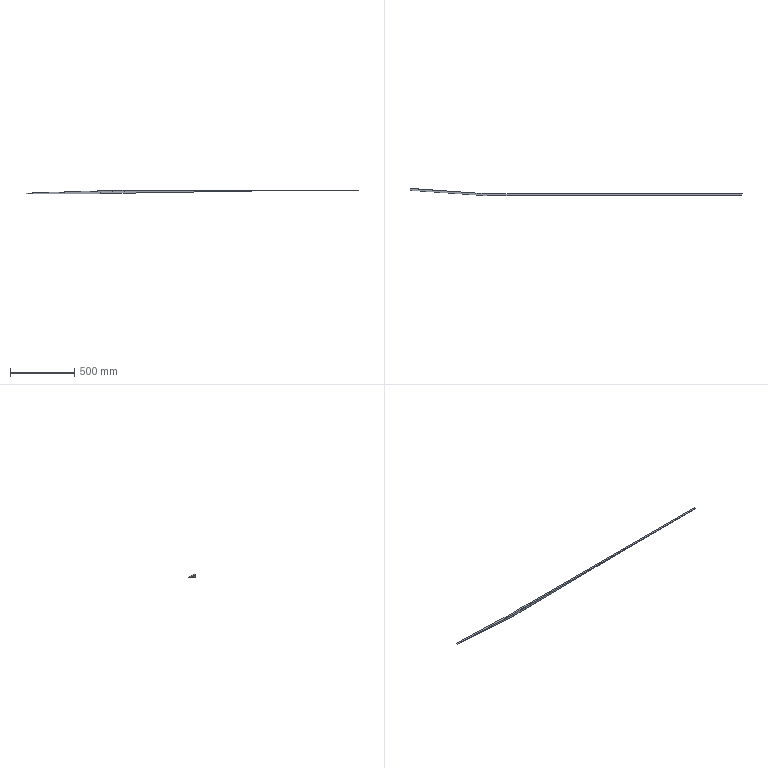Part | SolidWorks | features BaseBody 1 | 1 solid | 26 faces | box 2582 x 55.656 x 24.973 mm | volume 180184 mm3 | plane 26
STEP:
#1=CARTESIAN_POINT('',(2000.,-38.142,-0.6658));
#2=VERTEX_POINT('',#1);
#3=CARTESIAN_POINT('',(180.519,-38.128,-1.466));
#4=VERTEX_POINT('',#3);
#5=CARTESIAN_POINT('',(2000.,-38.142,-0.6658));
#6=DIRECTION('',(-1.,0.000007674,-0.0004396));
#7=VECTOR('',#6,1000.);
#8=LINE('',#5,#7);
#9=EDGE_CURVE('',#2,#4,#8,.T.);
#10=ORIENTED_EDGE('',*,*,#9,.F.);
#11=CARTESIAN_POINT('',(2000.,-23.141,-0.4373));
#12=VERTEX_POINT('',#11);
#13=CARTESIAN_POINT('',(2000.,-23.141,-0.4373));
#14=DIRECTION('',(-0.000000977,-0.9999,-0.01523));
#15=VECTOR('',#14,1000.);
#16=LINE('',#13,#15);
#17=EDGE_CURVE('',#12,#2,#16,.T.);
#18=ORIENTED_EDGE('',*,*,#17,.F.);
#19=CARTESIAN_POINT('',(180.519,-23.127,-1.237));
#20=VERTEX_POINT('',#19);
#21=CARTESIAN_POINT('',(180.519,-23.127,-1.237));
#22=DIRECTION('',(1.,-0.000007674,0.0004396));
#23=VECTOR('',#22,1000.);
#24=LINE('',#21,#23);
#25=EDGE_CURVE('',#20,#12,#24,.T.);
#26=ORIENTED_EDGE('',*,*,#25,.F.);
#27=CARTESIAN_POINT('',(180.519,-23.127,-1.237));
#28=DIRECTION('',(0.,0.9999,0.01523));
#29=VECTOR('',#28,1000.);
#30=LINE('',#27,#29);
#31=EDGE_CURVE('',#4,#20,#30,.T.);
#32=ORIENTED_EDGE('',*,*,#31,.F.);
#33=EDGE_LOOP('',(#10,#18,#26,#32));
#34=FACE_OUTER_BOUND('',#33,.T.);
#35=CARTESIAN_POINT('',(169.602,-38.22,-1.472));
#36=DIRECTION('',(0.0004397,0.01523,-0.9999));
#37=DIRECTION('',(0.,0.9999,0.01523));
#38=AXIS2_PLACEMENT_3D('',#35,#36,#37);
#39=PLANE('',#38);
#40=ADVANCED_FACE('',(#34),#39,.F.);
#41=CARTESIAN_POINT('',(90.17,-23.127,-1.237));
#42=VERTEX_POINT('',#41);
#43=CARTESIAN_POINT('',(135.344,-23.127,-1.237));
#44=DIRECTION('',(-1.,0.,0.));
#45=VECTOR('',#44,1000.);
#46=LINE('',#43,#45);
#47=EDGE_CURVE('',#20,#42,#46,.T.);
#48=ORIENTED_EDGE('',*,*,#47,.T.);
#49=CARTESIAN_POINT('',(90.17,-38.128,-1.466));
#50=VERTEX_POINT('',#49);
#51=CARTESIAN_POINT('',(90.17,-23.127,-1.237));
#52=DIRECTION('',(-0.00001304,-0.9999,-0.01523));
#53=VECTOR('',#52,1000.);
#54=LINE('',#51,#53);
#55=EDGE_CURVE('',#42,#50,#54,.T.);
#56=ORIENTED_EDGE('',*,*,#55,.T.);
#57=CARTESIAN_POINT('',(135.344,-38.128,-1.466));
#58=DIRECTION('',(1.,0.,0.));
#59=VECTOR('',#58,1000.);
#60=LINE('',#57,#59);
#61=EDGE_CURVE('',#50,#4,#60,.T.);
#62=ORIENTED_EDGE('',*,*,#61,.T.);
#63=ORIENTED_EDGE('',*,*,#31,.T.);
#64=EDGE_LOOP('',(#48,#56,#62,#63));
#65=FACE_OUTER_BOUND('',#64,.T.);
#66=CARTESIAN_POINT('',(89.628,-23.127,-1.237));
#67=DIRECTION('',(0.,-0.01523,0.9999));
#68=DIRECTION('',(0.,-0.9999,-0.01523));
#69=AXIS2_PLACEMENT_3D('',#66,#67,#68);
#70=PLANE('',#69);
#71=ADVANCED_FACE('',(#65),#70,.T.);
#72=CARTESIAN_POINT('',(180.528,-37.811,-22.266));
#73=VERTEX_POINT('',#72);
#74=CARTESIAN_POINT('',(180.519,-38.128,-1.466));
#75=DIRECTION('',(0.0004397,0.01523,-0.9999));
#76=VECTOR('',#75,1000.);
#77=LINE('',#74,#76);
#78=EDGE_CURVE('',#4,#73,#77,.T.);
#79=ORIENTED_EDGE('',*,*,#78,.T.);
#80=CARTESIAN_POINT('',(1223.587,-38.087,-4.207));
#81=VERTEX_POINT('',#80);
#82=CARTESIAN_POINT('',(180.528,-37.811,-22.266));
#83=DIRECTION('',(0.9999,-0.0002647,0.01731));
#84=VECTOR('',#83,1000.);
#85=LINE('',#82,#84);
#86=EDGE_CURVE('',#73,#81,#85,.T.);
#87=ORIENTED_EDGE('',*,*,#86,.T.);
#88=CARTESIAN_POINT('',(2000.001,-38.093,-3.865));
#89=VERTEX_POINT('',#88);
#90=CARTESIAN_POINT('',(1223.587,-38.087,-4.207));
#91=DIRECTION('',(1.,-0.000007674,0.0004396));
#92=VECTOR('',#91,1000.);
#93=LINE('',#90,#92);
#94=EDGE_CURVE('',#81,#89,#93,.T.);
#95=ORIENTED_EDGE('',*,*,#94,.T.);
#96=CARTESIAN_POINT('',(2000.001,-38.093,-3.865));
#97=DIRECTION('',(-0.0004395,-0.01523,0.9999));
#98=VECTOR('',#97,1000.);
#99=LINE('',#96,#98);
#100=EDGE_CURVE('',#89,#2,#99,.T.);
#101=ORIENTED_EDGE('',*,*,#100,.T.);
#102=ORIENTED_EDGE('',*,*,#9,.T.);
#103=EDGE_LOOP('',(#79,#87,#95,#101,#102));
#104=FACE_OUTER_BOUND('',#103,.T.);
#105=CARTESIAN_POINT('',(180.519,-38.14,-0.6657));
#106=DIRECTION('',(-0.000000977,-0.9999,-0.01523));
#107=DIRECTION('',(0.,0.01523,-0.9999));
#108=AXIS2_PLACEMENT_3D('',#105,#106,#107);
#109=PLANE('',#108);
#110=ADVANCED_FACE('',(#104),#109,.T.);
#111=CARTESIAN_POINT('',(2000.001,-23.092,-3.637));
#112=VERTEX_POINT('',#111);
#113=CARTESIAN_POINT('',(2000.001,-23.092,-3.637));
#114=DIRECTION('',(-0.0004397,-0.01523,0.9999));
#115=VECTOR('',#114,1000.);
#116=LINE('',#113,#115);
#117=EDGE_CURVE('',#112,#12,#116,.T.);
#118=ORIENTED_EDGE('',*,*,#117,.T.);
#119=ORIENTED_EDGE('',*,*,#17,.T.);
#120=ORIENTED_EDGE('',*,*,#100,.F.);
#121=CARTESIAN_POINT('',(2000.001,-38.093,-3.865));
#122=DIRECTION('',(0.000000977,0.9999,0.01523));
#123=VECTOR('',#122,1000.);
#124=LINE('',#121,#123);
#125=EDGE_CURVE('',#89,#112,#124,.T.);
#126=ORIENTED_EDGE('',*,*,#125,.T.);
#127=EDGE_LOOP('',(#118,#119,#120,#126));
#128=FACE_OUTER_BOUND('',#127,.T.);
#129=CARTESIAN_POINT('',(2000.,-38.232,-0.4167));
#130=DIRECTION('',(1.,-0.000007674,0.0004396));
#131=DIRECTION('',(0.0004396,0.,-1.));
#132=AXIS2_PLACEMENT_3D('',#129,#130,#131);
#133=PLANE('',#132);
#134=ADVANCED_FACE('',(#128),#133,.T.);
#135=ORIENTED_EDGE('',*,*,#117,.F.);
#136=CARTESIAN_POINT('',(180.52,-23.079,-4.437));
#137=VERTEX_POINT('',#136);
#138=CARTESIAN_POINT('',(2000.001,-23.092,-3.637));
#139=DIRECTION('',(-1.,0.000007674,-0.0004396));
#140=VECTOR('',#139,1000.);
#141=LINE('',#138,#140);
#142=EDGE_CURVE('',#112,#137,#141,.T.);
#143=ORIENTED_EDGE('',*,*,#142,.T.);
#144=CARTESIAN_POINT('',(180.52,-23.079,-4.437));
#145=DIRECTION('',(-0.0004396,-0.01523,0.9999));
#146=VECTOR('',#145,1000.);
#147=LINE('',#144,#146);
#148=EDGE_CURVE('',#137,#20,#147,.T.);
#149=ORIENTED_EDGE('',*,*,#148,.T.);
#150=ORIENTED_EDGE('',*,*,#25,.T.);
#151=EDGE_LOOP('',(#135,#143,#149,#150));
#152=FACE_OUTER_BOUND('',#151,.T.);
#153=CARTESIAN_POINT('',(169.602,-23.078,-4.461));
#154=DIRECTION('',(0.000000977,0.9999,0.01523));
#155=DIRECTION('',(0.,-0.01523,0.9999));
#156=AXIS2_PLACEMENT_3D('',#153,#154,#155);
#157=PLANE('',#156);
#158=ADVANCED_FACE('',(#152),#157,.T.);
#159=CARTESIAN_POINT('',(-5.976,-23.078,-4.291));
#160=VERTEX_POINT('',#159);
#161=CARTESIAN_POINT('',(-5.976,-23.078,-4.291));
#162=DIRECTION('',(0.9995,-0.0005096,0.03174));
#163=VECTOR('',#162,1000.);
#164=LINE('',#161,#163);
#165=EDGE_CURVE('',#160,#42,#164,.T.);
#166=ORIENTED_EDGE('',*,*,#165,.F.);
#167=CARTESIAN_POINT('',(-6.5,-38.079,-4.536));
#168=VERTEX_POINT('',#167);
#169=CARTESIAN_POINT('',(-6.5,-38.079,-4.536));
#170=DIRECTION('',(0.03491,0.9993,0.01633));
#171=VECTOR('',#170,1000.);
#172=LINE('',#169,#171);
#173=EDGE_CURVE('',#168,#160,#172,.T.);
#174=ORIENTED_EDGE('',*,*,#173,.F.);
#175=CARTESIAN_POINT('',(90.17,-38.128,-1.466));
#176=DIRECTION('',(-0.9995,0.0005096,-0.03174));
#177=VECTOR('',#176,1000.);
#178=LINE('',#175,#177);
#179=EDGE_CURVE('',#50,#168,#178,.T.);
#180=ORIENTED_EDGE('',*,*,#179,.F.);
#181=ORIENTED_EDGE('',*,*,#55,.F.);
#182=EDGE_LOOP('',(#166,#174,#180,#181));
#183=FACE_OUTER_BOUND('',#182,.T.);
#184=CARTESIAN_POINT('',(90.758,-38.218,-1.448));
#185=DIRECTION('',(0.03175,0.01522,-0.9994));
#186=DIRECTION('',(-0.9995,0.,-0.03175));
#187=AXIS2_PLACEMENT_3D('',#184,#185,#186);
#188=PLANE('',#187);
#189=ADVANCED_FACE('',(#183),#188,.F.);
#190=CARTESIAN_POINT('',(90.221,-23.079,-4.437));
#191=VERTEX_POINT('',#190);
#192=CARTESIAN_POINT('',(135.345,-23.079,-4.437));
#193=DIRECTION('',(1.,0.,0.));
#194=VECTOR('',#193,1000.);
#195=LINE('',#192,#194);
#196=EDGE_CURVE('',#191,#137,#195,.T.);
#197=ORIENTED_EDGE('',*,*,#196,.F.);
#198=CARTESIAN_POINT('',(90.17,-23.127,-1.237));
#199=DIRECTION('',(0.01588,0.01523,-0.9998));
#200=VECTOR('',#199,1000.);
#201=LINE('',#198,#200);
#202=EDGE_CURVE('',#42,#191,#201,.T.);
#203=ORIENTED_EDGE('',*,*,#202,.F.);
#204=ORIENTED_EDGE('',*,*,#47,.F.);
#205=ORIENTED_EDGE('',*,*,#148,.F.);
#206=EDGE_LOOP('',(#197,#203,#204,#205));
#207=FACE_OUTER_BOUND('',#206,.T.);
#208=CARTESIAN_POINT('',(89.628,-23.127,-1.237));
#209=DIRECTION('',(0.,-0.9999,-0.01523));
#210=DIRECTION('',(0.,0.01523,-0.9999));
#211=AXIS2_PLACEMENT_3D('',#208,#209,#210);
#212=PLANE('',#211);
#213=ADVANCED_FACE('',(#207),#212,.F.);
#214=ORIENTED_EDGE('',*,*,#61,.F.);
#215=CARTESIAN_POINT('',(90.5,-37.811,-22.266));
#216=VERTEX_POINT('',#215);
#217=CARTESIAN_POINT('',(90.5,-37.811,-22.266));
#218=DIRECTION('',(-0.01588,-0.01523,0.9998));
#219=VECTOR('',#218,1000.);
#220=LINE('',#217,#219);
#221=EDGE_CURVE('',#216,#50,#220,.T.);
#222=ORIENTED_EDGE('',*,*,#221,.F.);
#223=CARTESIAN_POINT('',(135.349,-37.811,-22.266));
#224=DIRECTION('',(-1.,0.,0.));
#225=VECTOR('',#224,1000.);
#226=LINE('',#223,#225);
#227=EDGE_CURVE('',#73,#216,#226,.T.);
#228=ORIENTED_EDGE('',*,*,#227,.F.);
#229=ORIENTED_EDGE('',*,*,#78,.F.);
#230=EDGE_LOOP('',(#214,#222,#228,#229));
#231=FACE_OUTER_BOUND('',#230,.T.);
#232=CARTESIAN_POINT('',(89.628,-37.811,-22.266));
#233=DIRECTION('',(0.,0.9999,0.01523));
#234=DIRECTION('',(0.,-0.01523,0.9999));
#235=AXIS2_PLACEMENT_3D('',#232,#233,#234);
#236=PLANE('',#235);
#237=ADVANCED_FACE('',(#231),#236,.F.);
#238=CARTESIAN_POINT('',(180.528,-34.611,-22.218));
#239=VERTEX_POINT('',#238);
#240=CARTESIAN_POINT('',(180.528,-37.811,-22.266));
#241=DIRECTION('',(0.,-0.9999,-0.01523));
#242=VECTOR('',#241,1000.);
#243=LINE('',#240,#242);
#244=EDGE_CURVE('',#239,#73,#243,.T.);
#245=ORIENTED_EDGE('',*,*,#244,.F.);
#246=CARTESIAN_POINT('',(1223.587,-34.887,-4.158));
#247=VERTEX_POINT('',#246);
#248=CARTESIAN_POINT('',(1223.587,-34.887,-4.158));
#249=DIRECTION('',(-0.9999,0.0002647,-0.01731));
#250=VECTOR('',#249,1000.);
#251=LINE('',#248,#250);
#252=EDGE_CURVE('',#247,#239,#251,.T.);
#253=ORIENTED_EDGE('',*,*,#252,.F.);
#254=CARTESIAN_POINT('',(1223.587,-38.088,-4.207));
#255=DIRECTION('',(0.,0.9999,0.01523));
#256=VECTOR('',#255,1000.);
#257=LINE('',#254,#256);
#258=EDGE_CURVE('',#81,#247,#257,.T.);
#259=ORIENTED_EDGE('',*,*,#258,.F.);
#260=ORIENTED_EDGE('',*,*,#86,.F.);
#261=EDGE_LOOP('',(#245,#253,#259,#260));
#262=FACE_OUTER_BOUND('',#261,.T.);
#263=CARTESIAN_POINT('',(174.27,-38.108,-22.379));
#264=DIRECTION('',(-0.01731,-0.01523,0.9997));
#265=DIRECTION('',(0.9999,0.,0.01732));
#266=AXIS2_PLACEMENT_3D('',#263,#264,#265);
#267=PLANE('',#266);
#268=ADVANCED_FACE('',(#262),#267,.F.);
#269=ORIENTED_EDGE('',*,*,#258,.T.);
#270=CARTESIAN_POINT('',(180.52,-34.879,-4.617));
#271=VERTEX_POINT('',#270);
#272=CARTESIAN_POINT('',(1223.587,-34.887,-4.158));
#273=DIRECTION('',(-1.,0.000007674,-0.0004396));
#274=VECTOR('',#273,1000.);
#275=LINE('',#272,#274);
#276=EDGE_CURVE('',#247,#271,#275,.T.);
#277=ORIENTED_EDGE('',*,*,#276,.T.);
#278=CARTESIAN_POINT('',(180.52,-38.081,-4.665));
#279=DIRECTION('',(0.,0.9999,0.01523));
#280=VECTOR('',#279,1000.);
#281=LINE('',#278,#280);
#282=EDGE_CURVE('',#271,#137,#281,.T.);
#283=ORIENTED_EDGE('',*,*,#282,.T.);
#284=ORIENTED_EDGE('',*,*,#142,.F.);
#285=ORIENTED_EDGE('',*,*,#125,.F.);
#286=ORIENTED_EDGE('',*,*,#94,.F.);
#287=EDGE_LOOP('',(#269,#277,#283,#284,#285,#286));
#288=FACE_OUTER_BOUND('',#287,.T.);
#289=CARTESIAN_POINT('',(180.52,-38.081,-4.665));
#290=DIRECTION('',(0.0004397,0.01523,-0.9999));
#291=DIRECTION('',(0.,0.9999,0.01523));
#292=AXIS2_PLACEMENT_3D('',#289,#290,#291);
#293=PLANE('',#292);
#294=ADVANCED_FACE('',(#288),#293,.T.);
#295=CARTESIAN_POINT('',(-5.875,-23.03,-7.489));
#296=VERTEX_POINT('',#295);
#297=CARTESIAN_POINT('',(90.221,-23.079,-4.437));
#298=DIRECTION('',(-0.9995,0.0005096,-0.03174));
#299=VECTOR('',#298,1000.);
#300=LINE('',#297,#299);
#301=EDGE_CURVE('',#191,#296,#300,.T.);
#302=ORIENTED_EDGE('',*,*,#301,.T.);
#303=CARTESIAN_POINT('',(-5.875,-23.03,-7.489));
#304=DIRECTION('',(-0.03175,-0.01522,0.9994));
#305=VECTOR('',#304,1000.);
#306=LINE('',#303,#305);
#307=EDGE_CURVE('',#296,#160,#306,.T.);
#308=ORIENTED_EDGE('',*,*,#307,.T.);
#309=ORIENTED_EDGE('',*,*,#165,.T.);
#310=ORIENTED_EDGE('',*,*,#202,.T.);
#311=EDGE_LOOP('',(#302,#308,#309,#310));
#312=FACE_OUTER_BOUND('',#311,.T.);
#313=CARTESIAN_POINT('',(-6.554,-23.029,-7.526));
#314=DIRECTION('',(0.00002607,0.9999,0.01523));
#315=DIRECTION('',(0.,-0.01523,0.9999));
#316=AXIS2_PLACEMENT_3D('',#313,#314,#315);
#317=PLANE('',#316);
#318=ADVANCED_FACE('',(#312),#317,.T.);
#319=CARTESIAN_POINT('',(-581.281,17.465,-21.951));
#320=VERTEX_POINT('',#319);
#321=CARTESIAN_POINT('',(-5.976,-23.078,-4.291));
#322=DIRECTION('',(-0.9971,0.07027,-0.03061));
#323=VECTOR('',#322,1000.);
#324=LINE('',#321,#323);
#325=EDGE_CURVE('',#160,#320,#324,.T.);
#326=ORIENTED_EDGE('',*,*,#325,.T.);
#327=CARTESIAN_POINT('',(-582.328,2.502,-22.213));
#328=VERTEX_POINT('',#327);
#329=CARTESIAN_POINT('',(-581.281,17.465,-21.951));
#330=DIRECTION('',(-0.06976,-0.9974,-0.01741));
#331=VECTOR('',#330,1000.);
#332=LINE('',#329,#331);
#333=EDGE_CURVE('',#320,#328,#332,.T.);
#334=ORIENTED_EDGE('',*,*,#333,.T.);
#335=CARTESIAN_POINT('',(-582.328,2.502,-22.213));
#336=DIRECTION('',(0.9971,-0.07027,0.03061));
#337=VECTOR('',#336,1000.);
#338=LINE('',#335,#337);
#339=EDGE_CURVE('',#328,#168,#338,.T.);
#340=ORIENTED_EDGE('',*,*,#339,.T.);
#341=ORIENTED_EDGE('',*,*,#173,.T.);
#342=EDGE_LOOP('',(#326,#334,#340,#341));
#343=FACE_OUTER_BOUND('',#342,.T.);
#344=CARTESIAN_POINT('',(-585.766,-38.412,-22.945));
#345=DIRECTION('',(-0.03175,-0.01522,0.9994));
#346=DIRECTION('',(0.9995,0.,0.03176));
#347=AXIS2_PLACEMENT_3D('',#344,#345,#346);
#348=PLANE('',#347);
#349=ADVANCED_FACE('',(#343),#348,.T.);
#350=ORIENTED_EDGE('',*,*,#179,.T.);
#351=CARTESIAN_POINT('',(-5.84,-37.762,-25.326));
#352=VERTEX_POINT('',#351);
#353=CARTESIAN_POINT('',(-6.5,-38.079,-4.536));
#354=DIRECTION('',(0.03175,0.01522,-0.9994));
#355=VECTOR('',#354,1000.);
#356=LINE('',#353,#355);
#357=EDGE_CURVE('',#168,#352,#356,.T.);
#358=ORIENTED_EDGE('',*,*,#357,.T.);
#359=CARTESIAN_POINT('',(-5.84,-37.762,-25.326));
#360=DIRECTION('',(0.9995,-0.0005096,0.03174));
#361=VECTOR('',#360,1000.);
#362=LINE('',#359,#361);
#363=EDGE_CURVE('',#352,#216,#362,.T.);
#364=ORIENTED_EDGE('',*,*,#363,.T.);
#365=ORIENTED_EDGE('',*,*,#221,.T.);
#366=EDGE_LOOP('',(#350,#358,#364,#365));
#367=FACE_OUTER_BOUND('',#366,.T.);
#368=CARTESIAN_POINT('',(-7.082,-38.127,-1.322));
#369=DIRECTION('',(-0.00002607,-0.9999,-0.01523));
#370=DIRECTION('',(0.,0.01523,-0.9999));
#371=AXIS2_PLACEMENT_3D('',#368,#369,#370);
#372=PLANE('',#371);
#373=ADVANCED_FACE('',(#367),#372,.T.);
#374=CARTESIAN_POINT('',(90.221,-34.879,-4.617));
#375=VERTEX_POINT('',#374);
#376=CARTESIAN_POINT('',(135.371,-34.879,-4.617));
#377=DIRECTION('',(1.,0.,0.));
#378=VECTOR('',#377,1000.);
#379=LINE('',#376,#378);
#380=EDGE_CURVE('',#375,#271,#379,.T.);
#381=ORIENTED_EDGE('',*,*,#380,.F.);
#382=CARTESIAN_POINT('',(90.221,-23.079,-4.437));
#383=DIRECTION('',(-0.00001304,-0.9999,-0.01523));
#384=VECTOR('',#383,1000.);
#385=LINE('',#382,#384);
#386=EDGE_CURVE('',#191,#375,#385,.T.);
#387=ORIENTED_EDGE('',*,*,#386,.F.);
#388=ORIENTED_EDGE('',*,*,#196,.T.);
#389=ORIENTED_EDGE('',*,*,#282,.F.);
#390=EDGE_LOOP('',(#381,#387,#388,#389));
#391=FACE_OUTER_BOUND('',#390,.T.);
#392=CARTESIAN_POINT('',(89.679,-23.079,-4.437));
#393=DIRECTION('',(0.,-0.01523,0.9999));
#394=DIRECTION('',(0.,-0.9999,-0.01523));
#395=AXIS2_PLACEMENT_3D('',#392,#393,#394);
#396=PLANE('',#395);
#397=ADVANCED_FACE('',(#391),#396,.F.);
#398=ORIENTED_EDGE('',*,*,#227,.T.);
#399=CARTESIAN_POINT('',(90.5,-34.611,-22.218));
#400=VERTEX_POINT('',#399);
#401=CARTESIAN_POINT('',(90.5,-37.811,-22.266));
#402=DIRECTION('',(0.00001302,0.9999,0.01523));
#403=VECTOR('',#402,1000.);
#404=LINE('',#401,#403);
#405=EDGE_CURVE('',#216,#400,#404,.T.);
#406=ORIENTED_EDGE('',*,*,#405,.T.);
#407=CARTESIAN_POINT('',(135.244,-34.611,-22.218));
#408=DIRECTION('',(1.,0.,0.));
#409=VECTOR('',#408,1000.);
#410=LINE('',#407,#409);
#411=EDGE_CURVE('',#400,#239,#410,.T.);
#412=ORIENTED_EDGE('',*,*,#411,.T.);
#413=ORIENTED_EDGE('',*,*,#244,.T.);
#414=EDGE_LOOP('',(#398,#406,#412,#413));
#415=FACE_OUTER_BOUND('',#414,.T.);
#416=CARTESIAN_POINT('',(89.96,-37.811,-22.266));
#417=DIRECTION('',(0.,0.01523,-0.9999));
#418=DIRECTION('',(0.,0.9999,0.01523));
#419=AXIS2_PLACEMENT_3D('',#416,#417,#418);
#420=PLANE('',#419);
#421=ADVANCED_FACE('',(#415),#420,.T.);
#422=ORIENTED_EDGE('',*,*,#252,.T.);
#423=CARTESIAN_POINT('',(180.52,-34.879,-4.617));
#424=DIRECTION('',(0.0004397,0.01523,-0.9999));
#425=VECTOR('',#424,1000.);
#426=LINE('',#423,#425);
#427=EDGE_CURVE('',#271,#239,#426,.T.);
#428=ORIENTED_EDGE('',*,*,#427,.F.);
#429=ORIENTED_EDGE('',*,*,#276,.F.);
#430=EDGE_LOOP('',(#422,#428,#429));
#431=FACE_OUTER_BOUND('',#430,.T.);
#432=CARTESIAN_POINT('',(174.262,-34.888,-4.05));
#433=DIRECTION('',(-0.000000977,-0.9999,-0.01523));
#434=DIRECTION('',(0.,0.01523,-0.9999));
#435=AXIS2_PLACEMENT_3D('',#432,#433,#434);
#436=PLANE('',#435);
#437=ADVANCED_FACE('',(#431),#436,.F.);
#438=CARTESIAN_POINT('',(-581.18,17.514,-25.149));
#439=VERTEX_POINT('',#438);
#440=CARTESIAN_POINT('',(-581.18,17.514,-25.149));
#441=DIRECTION('',(0.9971,-0.07027,0.03061));
#442=VECTOR('',#441,1000.);
#443=LINE('',#440,#442);
#444=EDGE_CURVE('',#439,#296,#443,.T.);
#445=ORIENTED_EDGE('',*,*,#444,.F.);
#446=CARTESIAN_POINT('',(-581.281,17.465,-21.951));
#447=DIRECTION('',(0.03175,0.01522,-0.9994));
#448=VECTOR('',#447,1000.);
#449=LINE('',#446,#448);
#450=EDGE_CURVE('',#320,#439,#449,.T.);
#451=ORIENTED_EDGE('',*,*,#450,.F.);
#452=ORIENTED_EDGE('',*,*,#325,.F.);
#453=ORIENTED_EDGE('',*,*,#307,.F.);
#454=EDGE_LOOP('',(#445,#451,#452,#453));
#455=FACE_OUTER_BOUND('',#454,.T.);
#456=CARTESIAN_POINT('',(-584.73,17.765,-25.275));
#457=DIRECTION('',(-0.06976,-0.9974,-0.01741));
#458=DIRECTION('',(0.9976,-0.06977,0.));
#459=AXIS2_PLACEMENT_3D('',#456,#457,#458);
#460=PLANE('',#459);
#461=ADVANCED_FACE('',(#455),#460,.F.);
#462=CARTESIAN_POINT('',(-6.287,-34.83,-7.681));
#463=VERTEX_POINT('',#462);
#464=CARTESIAN_POINT('',(90.221,-34.879,-4.617));
#465=DIRECTION('',(-0.9995,0.0005096,-0.03174));
#466=VECTOR('',#465,1000.);
#467=LINE('',#464,#466);
#468=EDGE_CURVE('',#375,#463,#467,.T.);
#469=ORIENTED_EDGE('',*,*,#468,.T.);
#470=CARTESIAN_POINT('',(-6.287,-34.83,-7.681));
#471=DIRECTION('',(0.03491,0.9993,0.01633));
#472=VECTOR('',#471,1000.);
#473=LINE('',#470,#472);
#474=EDGE_CURVE('',#463,#296,#473,.T.);
#475=ORIENTED_EDGE('',*,*,#474,.T.);
#476=ORIENTED_EDGE('',*,*,#301,.F.);
#477=ORIENTED_EDGE('',*,*,#386,.T.);
#478=EDGE_LOOP('',(#469,#475,#476,#477));
#479=FACE_OUTER_BOUND('',#478,.T.);
#480=CARTESIAN_POINT('',(90.806,-34.951,-4.599));
#481=DIRECTION('',(0.03175,0.01522,-0.9994));
#482=DIRECTION('',(-0.9995,0.,-0.03175));
#483=AXIS2_PLACEMENT_3D('',#480,#481,#482);
#484=PLANE('',#483);
#485=ADVANCED_FACE('',(#479),#484,.T.);
#486=CARTESIAN_POINT('',(-582.226,2.551,-25.411));
#487=VERTEX_POINT('',#486);
#488=CARTESIAN_POINT('',(-582.003,5.742,-25.355));
#489=VERTEX_POINT('',#488);
#490=CARTESIAN_POINT('',(-582.226,2.551,-25.411));
#491=DIRECTION('',(0.06976,0.9974,0.01741));
#492=VECTOR('',#491,1000.);
#493=LINE('',#490,#492);
#494=EDGE_CURVE('',#487,#489,#493,.T.);
#495=ORIENTED_EDGE('',*,*,#494,.F.);
#496=CARTESIAN_POINT('',(-582.328,2.502,-22.213));
#497=DIRECTION('',(0.03175,0.01522,-0.9994));
#498=VECTOR('',#497,1000.);
#499=LINE('',#496,#498);
#500=EDGE_CURVE('',#328,#487,#499,.T.);
#501=ORIENTED_EDGE('',*,*,#500,.F.);
#502=ORIENTED_EDGE('',*,*,#333,.F.);
#503=ORIENTED_EDGE('',*,*,#450,.T.);
#504=CARTESIAN_POINT('',(-582.003,5.742,-25.355));
#505=DIRECTION('',(0.06976,0.9974,0.01741));
#506=VECTOR('',#505,1000.);
#507=LINE('',#504,#506);
#508=EDGE_CURVE('',#489,#439,#507,.T.);
#509=ORIENTED_EDGE('',*,*,#508,.F.);
#510=EDGE_LOOP('',(#495,#501,#502,#503,#509));
#511=FACE_OUTER_BOUND('',#510,.T.);
#512=CARTESIAN_POINT('',(-582.23,2.495,-25.411));
#513=DIRECTION('',(0.9971,-0.07027,0.03061));
#514=DIRECTION('',(0.0703,0.9975,0.));
#515=AXIS2_PLACEMENT_3D('',#512,#513,#514);
#516=PLANE('',#515);
#517=ADVANCED_FACE('',(#511),#516,.F.);
#518=CARTESIAN_POINT('',(-5.951,-37.754,-25.329));
#519=VERTEX_POINT('',#518);
#520=CARTESIAN_POINT('',(-5.951,-37.754,-25.329));
#521=DIRECTION('',(-0.9976,0.06977,-0.0001404));
#522=VECTOR('',#521,1000.);
#523=LINE('',#520,#522);
#524=EDGE_CURVE('',#519,#487,#523,.T.);
#525=ORIENTED_EDGE('',*,*,#524,.F.);
#526=CARTESIAN_POINT('',(-5.84,-37.762,-25.326));
#527=DIRECTION('',(-0.9971,0.07027,-0.03061));
#528=VECTOR('',#527,1000.);
#529=LINE('',#526,#528);
#530=EDGE_CURVE('',#352,#519,#529,.T.);
#531=ORIENTED_EDGE('',*,*,#530,.F.);
#532=ORIENTED_EDGE('',*,*,#357,.F.);
#533=ORIENTED_EDGE('',*,*,#339,.F.);
#534=ORIENTED_EDGE('',*,*,#500,.T.);
#535=EDGE_LOOP('',(#525,#531,#532,#533,#534));
#536=FACE_OUTER_BOUND('',#535,.T.);
#537=CARTESIAN_POINT('',(-5.84,-37.76,-25.411));
#538=DIRECTION('',(0.06976,0.9974,0.01741));
#539=DIRECTION('',(-0.9976,0.06977,0.));
#540=AXIS2_PLACEMENT_3D('',#537,#538,#539);
#541=PLANE('',#540);
#542=ADVANCED_FACE('',(#536),#541,.F.);
#543=ORIENTED_EDGE('',*,*,#363,.F.);
#544=ORIENTED_EDGE('',*,*,#530,.T.);
#545=CARTESIAN_POINT('',(-5.728,-34.562,-25.274));
#546=VERTEX_POINT('',#545);
#547=CARTESIAN_POINT('',(-5.951,-37.754,-25.329));
#548=DIRECTION('',(0.06976,0.9974,0.01741));
#549=VECTOR('',#548,1000.);
#550=LINE('',#547,#549);
#551=EDGE_CURVE('',#519,#546,#550,.T.);
#552=ORIENTED_EDGE('',*,*,#551,.T.);
#553=CARTESIAN_POINT('',(90.5,-34.611,-22.218));
#554=DIRECTION('',(-0.9995,0.0005096,-0.03174));
#555=VECTOR('',#554,1000.);
#556=LINE('',#553,#555);
#557=EDGE_CURVE('',#400,#546,#556,.T.);
#558=ORIENTED_EDGE('',*,*,#557,.F.);
#559=ORIENTED_EDGE('',*,*,#405,.F.);
#560=EDGE_LOOP('',(#543,#544,#552,#558,#559));
#561=FACE_OUTER_BOUND('',#560,.T.);
#562=CARTESIAN_POINT('',(-6.418,-37.83,-25.345));
#563=DIRECTION('',(-0.03175,-0.01522,0.9994));
#564=DIRECTION('',(0.9995,0.,0.03175));
#565=AXIS2_PLACEMENT_3D('',#562,#563,#564);
#566=PLANE('',#565);
#567=ADVANCED_FACE('',(#561),#566,.F.);
#568=ORIENTED_EDGE('',*,*,#411,.F.);
#569=CARTESIAN_POINT('',(90.5,-34.611,-22.218));
#570=DIRECTION('',(-0.01588,-0.01523,0.9998));
#571=VECTOR('',#570,1000.);
#572=LINE('',#569,#571);
#573=EDGE_CURVE('',#400,#375,#572,.T.);
#574=ORIENTED_EDGE('',*,*,#573,.T.);
#575=ORIENTED_EDGE('',*,*,#380,.T.);
#576=ORIENTED_EDGE('',*,*,#427,.T.);
#577=EDGE_LOOP('',(#568,#574,#575,#576));
#578=FACE_OUTER_BOUND('',#577,.T.);
#579=CARTESIAN_POINT('',(89.679,-34.611,-22.218));
#580=DIRECTION('',(0.,0.9999,0.01523));
#581=DIRECTION('',(0.,-0.01523,0.9999));
#582=AXIS2_PLACEMENT_3D('',#579,#580,#581);
#583=PLANE('',#582);
#584=ADVANCED_FACE('',(#578),#583,.T.);
#585=CARTESIAN_POINT('',(-582.003,5.742,-25.355));
#586=DIRECTION('',(0.9971,-0.07027,0.03061));
#587=VECTOR('',#586,1000.);
#588=LINE('',#585,#587);
#589=EDGE_CURVE('',#489,#463,#588,.T.);
#590=ORIENTED_EDGE('',*,*,#589,.F.);
#591=ORIENTED_EDGE('',*,*,#508,.T.);
#592=ORIENTED_EDGE('',*,*,#444,.T.);
#593=ORIENTED_EDGE('',*,*,#474,.F.);
#594=EDGE_LOOP('',(#590,#591,#592,#593));
#595=FACE_OUTER_BOUND('',#594,.T.);
#596=CARTESIAN_POINT('',(-585.44,-35.144,-26.087));
#597=DIRECTION('',(-0.03175,-0.01522,0.9994));
#598=DIRECTION('',(0.9995,0.,0.03176));
#599=AXIS2_PLACEMENT_3D('',#596,#597,#598);
#600=PLANE('',#599);
#601=ADVANCED_FACE('',(#595),#600,.F.);
#602=ORIENTED_EDGE('',*,*,#557,.T.);
#603=CARTESIAN_POINT('',(-6.287,-34.83,-7.681));
#604=DIRECTION('',(0.03175,0.01522,-0.9994));
#605=VECTOR('',#604,1000.);
#606=LINE('',#603,#605);
#607=EDGE_CURVE('',#463,#546,#606,.T.);
#608=ORIENTED_EDGE('',*,*,#607,.F.);
#609=ORIENTED_EDGE('',*,*,#468,.F.);
#610=ORIENTED_EDGE('',*,*,#573,.F.);
#611=EDGE_LOOP('',(#602,#608,#609,#610));
#612=FACE_OUTER_BOUND('',#611,.T.);
#613=CARTESIAN_POINT('',(-6.868,-34.879,-4.493));
#614=DIRECTION('',(-0.00002607,-0.9999,-0.01523));
#615=DIRECTION('',(0.,0.01523,-0.9999));
#616=AXIS2_PLACEMENT_3D('',#613,#614,#615);
#617=PLANE('',#616);
#618=ADVANCED_FACE('',(#612),#617,.F.);
#619=CARTESIAN_POINT('',(-5.728,-34.562,-25.274));
#620=DIRECTION('',(-0.9976,0.06977,-0.0001404));
#621=VECTOR('',#620,1000.);
#622=LINE('',#619,#621);
#623=EDGE_CURVE('',#546,#489,#622,.T.);
#624=ORIENTED_EDGE('',*,*,#623,.F.);
#625=ORIENTED_EDGE('',*,*,#551,.F.);
#626=ORIENTED_EDGE('',*,*,#524,.T.);
#627=ORIENTED_EDGE('',*,*,#494,.T.);
#628=EDGE_LOOP('',(#624,#625,#626,#627));
#629=FACE_OUTER_BOUND('',#628,.T.);
#630=CARTESIAN_POINT('',(-585.685,6.003,-25.355));
#631=DIRECTION('',(-0.001355,-0.01736,0.9998));
#632=DIRECTION('',(0.,-0.9998,-0.01736));
#633=AXIS2_PLACEMENT_3D('',#630,#631,#632);
#634=PLANE('',#633);
#635=ADVANCED_FACE('',(#629),#634,.F.);
#636=ORIENTED_EDGE('',*,*,#589,.T.);
#637=ORIENTED_EDGE('',*,*,#607,.T.);
#638=ORIENTED_EDGE('',*,*,#623,.T.);
#639=EDGE_LOOP('',(#636,#637,#638));
#640=FACE_OUTER_BOUND('',#639,.T.);
#641=CARTESIAN_POINT('',(-2.27,-34.801,-25.461));
#642=DIRECTION('',(0.06976,0.9974,0.01741));
#643=DIRECTION('',(-0.9976,0.06977,0.));
#644=AXIS2_PLACEMENT_3D('',#641,#642,#643);
#645=PLANE('',#644);
#646=ADVANCED_FACE('',(#640),#645,.T.);
#647=CLOSED_SHELL('',(#40,#71,#110,#134,#158,#189,#213,#237,#268,#294,#318,#349,#373,#397,#421,#437,#461,#485,#517,#542,#567,#584,#601,#618,#635,#646));
#648=MANIFOLD_SOLID_BREP('',#647);
#649=CARTESIAN_POINT('',(0.,0.,0.));
#650=DIRECTION('',(0.,0.,1.));
#651=DIRECTION('',(1.,0.,0.));
#652=AXIS2_PLACEMENT_3D('',#649,#650,#651);
#653=(LENGTH_UNIT()NAMED_UNIT(*)SI_UNIT(.MILLI.,.METRE.));
#654=UNCERTAINTY_MEASURE_WITH_UNIT(LENGTH_MEASURE(0.00001),#653,'','');
#655=(NAMED_UNIT(*)PLANE_ANGLE_UNIT()SI_UNIT($,.RADIAN.));
#656=(NAMED_UNIT(*)SI_UNIT($,.STERADIAN.)SOLID_ANGLE_UNIT());
#657=(GEOMETRIC_REPRESENTATION_CONTEXT(3)GLOBAL_UNCERTAINTY_ASSIGNED_CONTEXT((#654))GLOBAL_UNIT_ASSIGNED_CONTEXT((#653,#655,#656))REPRESENTATION_CONTEXT('',''));
#658=ADVANCED_BREP_SHAPE_REPRESENTATION('',(#648,#652),#657);